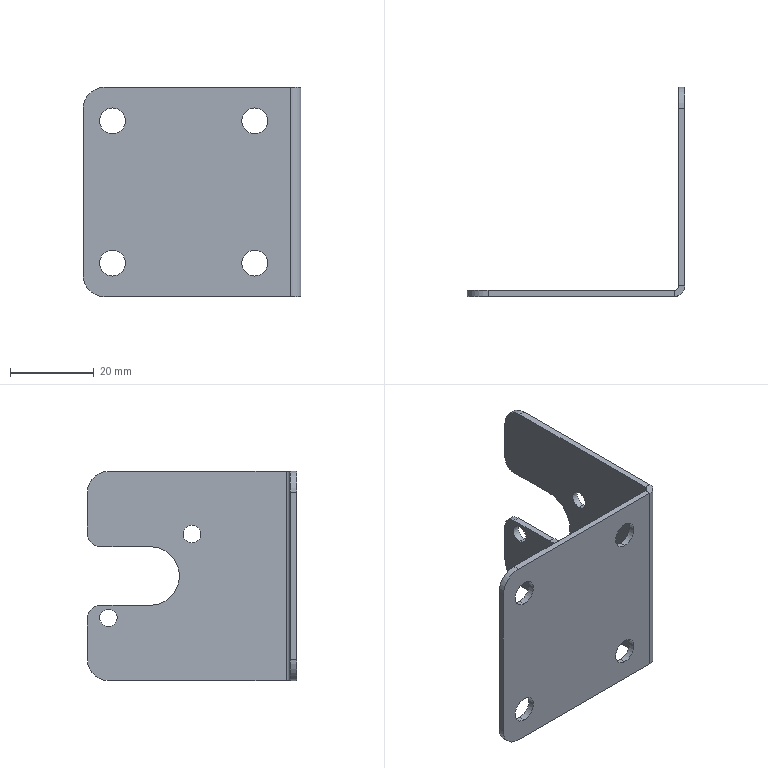Part | SolidWorks | features Fillet 2, HoleWzd 2, ICE 2, EdgeFlange 1, FlatPattern 1, SMBaseFlange 1, SheetMetal 1 | 1 solid | 36 faces | box 52 x 50 x 50 mm | volume 6790 mm3 | cylinder 21 | plane 15 | commonest cylinder face diameters 6.2 x8 4.2 x4 10 x4 6 x2 2 x1 5 x1
STEP:
#1=CARTESIAN_POINT('',(24.5,43.5,-12.1));
#2=VERTEX_POINT('',#1);
#3=CARTESIAN_POINT('',(24.5,43.5,-7.9));
#4=VERTEX_POINT('',#3);
#5=CARTESIAN_POINT('',(24.5,43.5,-10.));
#6=DIRECTION('',(-1.,0.,0.));
#7=DIRECTION('',(0.,-1.,0.));
#8=AXIS2_PLACEMENT_3D('',#5,#6,#7);
#9=CIRCLE('',#8,2.1);
#10=EDGE_CURVE('',#2,#4,#9,.T.);
#11=ORIENTED_EDGE('',*,*,#10,.T.);
#12=CARTESIAN_POINT('',(26.,43.5,-7.9));
#13=VERTEX_POINT('',#12);
#14=CARTESIAN_POINT('',(26.,43.5,-7.9));
#15=DIRECTION('',(1.,0.,0.));
#16=VECTOR('',#15,1000.);
#17=LINE('',#14,#16);
#18=EDGE_CURVE('',#4,#13,#17,.T.);
#19=ORIENTED_EDGE('',*,*,#18,.T.);
#20=CARTESIAN_POINT('',(26.,43.5,-12.1));
#21=VERTEX_POINT('',#20);
#22=CARTESIAN_POINT('',(26.,43.5,-10.));
#23=DIRECTION('',(1.,0.,0.));
#24=DIRECTION('',(0.,0.,-1.));
#25=AXIS2_PLACEMENT_3D('',#22,#23,#24);
#26=CIRCLE('',#25,2.1);
#27=EDGE_CURVE('',#13,#21,#26,.T.);
#28=ORIENTED_EDGE('',*,*,#27,.T.);
#29=CARTESIAN_POINT('',(26.,43.5,-12.1));
#30=DIRECTION('',(1.,0.,0.));
#31=VECTOR('',#30,1000.);
#32=LINE('',#29,#31);
#33=EDGE_CURVE('',#2,#21,#32,.T.);
#34=ORIENTED_EDGE('',*,*,#33,.F.);
#35=EDGE_LOOP('',(#11,#19,#28,#34));
#36=FACE_OUTER_BOUND('',#35,.T.);
#37=CARTESIAN_POINT('',(26.,43.5,-10.));
#38=DIRECTION('',(1.,0.,0.));
#39=DIRECTION('',(0.,0.,-1.));
#40=AXIS2_PLACEMENT_3D('',#37,#38,#39);
#41=CYLINDRICAL_SURFACE('',#40,2.1);
#42=ADVANCED_FACE('',(#36),#41,.F.);
#43=CARTESIAN_POINT('',(24.5,23.5,7.9));
#44=VERTEX_POINT('',#43);
#45=CARTESIAN_POINT('',(24.5,23.5,12.1));
#46=VERTEX_POINT('',#45);
#47=CARTESIAN_POINT('',(24.5,23.5,10.));
#48=DIRECTION('',(-1.,0.,0.));
#49=DIRECTION('',(0.,-1.,0.));
#50=AXIS2_PLACEMENT_3D('',#47,#48,#49);
#51=CIRCLE('',#50,2.1);
#52=EDGE_CURVE('',#44,#46,#51,.T.);
#53=ORIENTED_EDGE('',*,*,#52,.T.);
#54=CARTESIAN_POINT('',(26.,23.5,12.1));
#55=VERTEX_POINT('',#54);
#56=CARTESIAN_POINT('',(26.,23.5,12.1));
#57=DIRECTION('',(1.,0.,0.));
#58=VECTOR('',#57,1000.);
#59=LINE('',#56,#58);
#60=EDGE_CURVE('',#46,#55,#59,.T.);
#61=ORIENTED_EDGE('',*,*,#60,.T.);
#62=CARTESIAN_POINT('',(26.,23.5,7.9));
#63=VERTEX_POINT('',#62);
#64=CARTESIAN_POINT('',(26.,23.5,10.));
#65=DIRECTION('',(1.,0.,0.));
#66=DIRECTION('',(0.,0.,-1.));
#67=AXIS2_PLACEMENT_3D('',#64,#65,#66);
#68=CIRCLE('',#67,2.1);
#69=EDGE_CURVE('',#55,#63,#68,.T.);
#70=ORIENTED_EDGE('',*,*,#69,.T.);
#71=CARTESIAN_POINT('',(26.,23.5,7.9));
#72=DIRECTION('',(1.,0.,0.));
#73=VECTOR('',#72,1000.);
#74=LINE('',#71,#73);
#75=EDGE_CURVE('',#44,#63,#74,.T.);
#76=ORIENTED_EDGE('',*,*,#75,.F.);
#77=EDGE_LOOP('',(#53,#61,#70,#76));
#78=FACE_OUTER_BOUND('',#77,.T.);
#79=CARTESIAN_POINT('',(26.,23.5,10.));
#80=DIRECTION('',(1.,0.,0.));
#81=DIRECTION('',(0.,0.,-1.));
#82=AXIS2_PLACEMENT_3D('',#79,#80,#81);
#83=CYLINDRICAL_SURFACE('',#82,2.1);
#84=ADVANCED_FACE('',(#78),#83,.F.);
#85=CARTESIAN_POINT('',(-19.,-1.5,-13.9));
#86=VERTEX_POINT('',#85);
#87=CARTESIAN_POINT('',(-19.,-1.5,-20.1));
#88=VERTEX_POINT('',#87);
#89=CARTESIAN_POINT('',(-19.,-1.5,-17.));
#90=DIRECTION('',(0.,-1.,0.));
#91=DIRECTION('',(0.,0.,-1.));
#92=AXIS2_PLACEMENT_3D('',#89,#90,#91);
#93=CIRCLE('',#92,3.1);
#94=EDGE_CURVE('',#86,#88,#93,.T.);
#95=ORIENTED_EDGE('',*,*,#94,.T.);
#96=CARTESIAN_POINT('',(-19.,0.,-20.1));
#97=VERTEX_POINT('',#96);
#98=CARTESIAN_POINT('',(-19.,0.,-20.1));
#99=DIRECTION('',(0.,1.,0.));
#100=VECTOR('',#99,1000.);
#101=LINE('',#98,#100);
#102=EDGE_CURVE('',#88,#97,#101,.T.);
#103=ORIENTED_EDGE('',*,*,#102,.T.);
#104=CARTESIAN_POINT('',(-19.,0.,-13.9));
#105=VERTEX_POINT('',#104);
#106=CARTESIAN_POINT('',(-19.,0.,-17.));
#107=DIRECTION('',(0.,1.,0.));
#108=DIRECTION('',(0.,0.,1.));
#109=AXIS2_PLACEMENT_3D('',#106,#107,#108);
#110=CIRCLE('',#109,3.1);
#111=EDGE_CURVE('',#97,#105,#110,.T.);
#112=ORIENTED_EDGE('',*,*,#111,.T.);
#113=CARTESIAN_POINT('',(-19.,0.,-13.9));
#114=DIRECTION('',(0.,1.,0.));
#115=VECTOR('',#114,1000.);
#116=LINE('',#113,#115);
#117=EDGE_CURVE('',#86,#105,#116,.T.);
#118=ORIENTED_EDGE('',*,*,#117,.F.);
#119=EDGE_LOOP('',(#95,#103,#112,#118));
#120=FACE_OUTER_BOUND('',#119,.T.);
#121=CARTESIAN_POINT('',(-19.,0.,-17.));
#122=DIRECTION('',(0.,1.,0.));
#123=DIRECTION('',(0.,0.,1.));
#124=AXIS2_PLACEMENT_3D('',#121,#122,#123);
#125=CYLINDRICAL_SURFACE('',#124,3.1);
#126=ADVANCED_FACE('',(#120),#125,.F.);
#127=CARTESIAN_POINT('',(15.,-1.5,20.1));
#128=VERTEX_POINT('',#127);
#129=CARTESIAN_POINT('',(15.,-1.5,13.9));
#130=VERTEX_POINT('',#129);
#131=CARTESIAN_POINT('',(15.,-1.5,17.));
#132=DIRECTION('',(0.,-1.,0.));
#133=DIRECTION('',(0.,0.,-1.));
#134=AXIS2_PLACEMENT_3D('',#131,#132,#133);
#135=CIRCLE('',#134,3.1);
#136=EDGE_CURVE('',#128,#130,#135,.T.);
#137=ORIENTED_EDGE('',*,*,#136,.T.);
#138=CARTESIAN_POINT('',(15.,0.,13.9));
#139=VERTEX_POINT('',#138);
#140=CARTESIAN_POINT('',(15.,0.,13.9));
#141=DIRECTION('',(0.,1.,0.));
#142=VECTOR('',#141,1000.);
#143=LINE('',#140,#142);
#144=EDGE_CURVE('',#130,#139,#143,.T.);
#145=ORIENTED_EDGE('',*,*,#144,.T.);
#146=CARTESIAN_POINT('',(15.,0.,20.1));
#147=VERTEX_POINT('',#146);
#148=CARTESIAN_POINT('',(15.,0.,17.));
#149=DIRECTION('',(0.,1.,0.));
#150=DIRECTION('',(0.,0.,1.));
#151=AXIS2_PLACEMENT_3D('',#148,#149,#150);
#152=CIRCLE('',#151,3.1);
#153=EDGE_CURVE('',#139,#147,#152,.T.);
#154=ORIENTED_EDGE('',*,*,#153,.T.);
#155=CARTESIAN_POINT('',(15.,0.,20.1));
#156=DIRECTION('',(0.,1.,0.));
#157=VECTOR('',#156,1000.);
#158=LINE('',#155,#157);
#159=EDGE_CURVE('',#128,#147,#158,.T.);
#160=ORIENTED_EDGE('',*,*,#159,.F.);
#161=EDGE_LOOP('',(#137,#145,#154,#160));
#162=FACE_OUTER_BOUND('',#161,.T.);
#163=CARTESIAN_POINT('',(15.,0.,17.));
#164=DIRECTION('',(0.,1.,0.));
#165=DIRECTION('',(0.,0.,1.));
#166=AXIS2_PLACEMENT_3D('',#163,#164,#165);
#167=CYLINDRICAL_SURFACE('',#166,3.1);
#168=ADVANCED_FACE('',(#162),#167,.F.);
#169=CARTESIAN_POINT('',(-19.,-1.5,20.1));
#170=VERTEX_POINT('',#169);
#171=CARTESIAN_POINT('',(-19.,-1.5,13.9));
#172=VERTEX_POINT('',#171);
#173=CARTESIAN_POINT('',(-19.,-1.5,17.));
#174=DIRECTION('',(0.,-1.,0.));
#175=DIRECTION('',(0.,0.,-1.));
#176=AXIS2_PLACEMENT_3D('',#173,#174,#175);
#177=CIRCLE('',#176,3.1);
#178=EDGE_CURVE('',#170,#172,#177,.T.);
#179=ORIENTED_EDGE('',*,*,#178,.T.);
#180=CARTESIAN_POINT('',(-19.,0.,13.9));
#181=VERTEX_POINT('',#180);
#182=CARTESIAN_POINT('',(-19.,0.,13.9));
#183=DIRECTION('',(0.,1.,0.));
#184=VECTOR('',#183,1000.);
#185=LINE('',#182,#184);
#186=EDGE_CURVE('',#172,#181,#185,.T.);
#187=ORIENTED_EDGE('',*,*,#186,.T.);
#188=CARTESIAN_POINT('',(-19.,0.,20.1));
#189=VERTEX_POINT('',#188);
#190=CARTESIAN_POINT('',(-19.,0.,17.));
#191=DIRECTION('',(0.,1.,0.));
#192=DIRECTION('',(0.,0.,1.));
#193=AXIS2_PLACEMENT_3D('',#190,#191,#192);
#194=CIRCLE('',#193,3.1);
#195=EDGE_CURVE('',#181,#189,#194,.T.);
#196=ORIENTED_EDGE('',*,*,#195,.T.);
#197=CARTESIAN_POINT('',(-19.,0.,20.1));
#198=DIRECTION('',(0.,1.,0.));
#199=VECTOR('',#198,1000.);
#200=LINE('',#197,#199);
#201=EDGE_CURVE('',#170,#189,#200,.T.);
#202=ORIENTED_EDGE('',*,*,#201,.F.);
#203=EDGE_LOOP('',(#179,#187,#196,#202));
#204=FACE_OUTER_BOUND('',#203,.T.);
#205=CARTESIAN_POINT('',(-19.,0.,17.));
#206=DIRECTION('',(0.,1.,0.));
#207=DIRECTION('',(0.,0.,1.));
#208=AXIS2_PLACEMENT_3D('',#205,#206,#207);
#209=CYLINDRICAL_SURFACE('',#208,3.1);
#210=ADVANCED_FACE('',(#204),#209,.F.);
#211=CARTESIAN_POINT('',(15.,-1.5,-13.9));
#212=VERTEX_POINT('',#211);
#213=CARTESIAN_POINT('',(15.,-1.5,-20.1));
#214=VERTEX_POINT('',#213);
#215=CARTESIAN_POINT('',(15.,-1.5,-17.));
#216=DIRECTION('',(0.,-1.,0.));
#217=DIRECTION('',(0.,0.,-1.));
#218=AXIS2_PLACEMENT_3D('',#215,#216,#217);
#219=CIRCLE('',#218,3.1);
#220=EDGE_CURVE('',#212,#214,#219,.T.);
#221=ORIENTED_EDGE('',*,*,#220,.T.);
#222=CARTESIAN_POINT('',(15.,0.,-20.1));
#223=VERTEX_POINT('',#222);
#224=CARTESIAN_POINT('',(15.,0.,-20.1));
#225=DIRECTION('',(0.,1.,0.));
#226=VECTOR('',#225,1000.);
#227=LINE('',#224,#226);
#228=EDGE_CURVE('',#214,#223,#227,.T.);
#229=ORIENTED_EDGE('',*,*,#228,.T.);
#230=CARTESIAN_POINT('',(15.,0.,-13.9));
#231=VERTEX_POINT('',#230);
#232=CARTESIAN_POINT('',(15.,0.,-17.));
#233=DIRECTION('',(0.,1.,0.));
#234=DIRECTION('',(0.,0.,1.));
#235=AXIS2_PLACEMENT_3D('',#232,#233,#234);
#236=CIRCLE('',#235,3.1);
#237=EDGE_CURVE('',#223,#231,#236,.T.);
#238=ORIENTED_EDGE('',*,*,#237,.T.);
#239=CARTESIAN_POINT('',(15.,0.,-13.9));
#240=DIRECTION('',(0.,1.,0.));
#241=VECTOR('',#240,1000.);
#242=LINE('',#239,#241);
#243=EDGE_CURVE('',#212,#231,#242,.T.);
#244=ORIENTED_EDGE('',*,*,#243,.F.);
#245=EDGE_LOOP('',(#221,#229,#238,#244));
#246=FACE_OUTER_BOUND('',#245,.T.);
#247=CARTESIAN_POINT('',(15.,0.,-17.));
#248=DIRECTION('',(0.,1.,0.));
#249=DIRECTION('',(0.,0.,1.));
#250=AXIS2_PLACEMENT_3D('',#247,#248,#249);
#251=CYLINDRICAL_SURFACE('',#250,3.1);
#252=ADVANCED_FACE('',(#246),#251,.F.);
#253=CARTESIAN_POINT('',(26.,23.5,10.));
#254=DIRECTION('',(1.,0.,0.));
#255=DIRECTION('',(0.,0.,-1.));
#256=AXIS2_PLACEMENT_3D('',#253,#254,#255);
#257=CIRCLE('',#256,2.1);
#258=EDGE_CURVE('',#63,#55,#257,.T.);
#259=ORIENTED_EDGE('',*,*,#258,.F.);
#260=ORIENTED_EDGE('',*,*,#69,.F.);
#261=EDGE_LOOP('',(#259,#260));
#262=FACE_BOUND('',#261,.T.);
#263=CARTESIAN_POINT('',(26.,43.5,-10.));
#264=DIRECTION('',(1.,0.,0.));
#265=DIRECTION('',(0.,0.,-1.));
#266=AXIS2_PLACEMENT_3D('',#263,#264,#265);
#267=CIRCLE('',#266,2.1);
#268=EDGE_CURVE('',#21,#13,#267,.T.);
#269=ORIENTED_EDGE('',*,*,#268,.F.);
#270=ORIENTED_EDGE('',*,*,#27,.F.);
#271=EDGE_LOOP('',(#269,#270));
#272=FACE_BOUND('',#271,.T.);
#273=CARTESIAN_POINT('',(26.,33.5,7.));
#274=VERTEX_POINT('',#273);
#275=CARTESIAN_POINT('',(26.,45.5,7.));
#276=VERTEX_POINT('',#275);
#277=CARTESIAN_POINT('',(26.,0.,7.));
#278=DIRECTION('',(0.,1.,0.));
#279=VECTOR('',#278,1000.);
#280=LINE('',#277,#279);
#281=EDGE_CURVE('',#274,#276,#280,.T.);
#282=ORIENTED_EDGE('',*,*,#281,.T.);
#283=CARTESIAN_POINT('',(26.,48.5,10.));
#284=VERTEX_POINT('',#283);
#285=CARTESIAN_POINT('',(26.,45.5,10.));
#286=DIRECTION('',(1.,0.,0.));
#287=DIRECTION('',(0.,-1.,0.));
#288=AXIS2_PLACEMENT_3D('',#285,#286,#287);
#289=CIRCLE('',#288,3.);
#290=EDGE_CURVE('',#276,#284,#289,.T.);
#291=ORIENTED_EDGE('',*,*,#290,.T.);
#292=CARTESIAN_POINT('',(26.,48.5,20.));
#293=VERTEX_POINT('',#292);
#294=CARTESIAN_POINT('',(26.,48.5,0.));
#295=DIRECTION('',(0.,0.,1.));
#296=VECTOR('',#295,1000.);
#297=LINE('',#294,#296);
#298=EDGE_CURVE('',#284,#293,#297,.T.);
#299=ORIENTED_EDGE('',*,*,#298,.T.);
#300=CARTESIAN_POINT('',(26.,43.5,25.));
#301=VERTEX_POINT('',#300);
#302=CARTESIAN_POINT('',(26.,43.5,20.));
#303=DIRECTION('',(1.,0.,0.));
#304=DIRECTION('',(0.,-1.,0.));
#305=AXIS2_PLACEMENT_3D('',#302,#303,#304);
#306=CIRCLE('',#305,5.);
#307=EDGE_CURVE('',#293,#301,#306,.T.);
#308=ORIENTED_EDGE('',*,*,#307,.T.);
#309=CARTESIAN_POINT('',(26.,1.,25.));
#310=VERTEX_POINT('',#309);
#311=CARTESIAN_POINT('',(26.,0.,25.));
#312=DIRECTION('',(0.,-1.,0.));
#313=VECTOR('',#312,1000.);
#314=LINE('',#311,#313);
#315=EDGE_CURVE('',#301,#310,#314,.T.);
#316=ORIENTED_EDGE('',*,*,#315,.T.);
#317=CARTESIAN_POINT('',(26.,1.,-25.));
#318=VERTEX_POINT('',#317);
#319=CARTESIAN_POINT('',(26.,1.,25.));
#320=DIRECTION('',(0.,0.,1.));
#321=VECTOR('',#320,1000.);
#322=LINE('',#319,#321);
#323=EDGE_CURVE('',#318,#310,#322,.T.);
#324=ORIENTED_EDGE('',*,*,#323,.F.);
#325=CARTESIAN_POINT('',(26.,43.5,-25.));
#326=VERTEX_POINT('',#325);
#327=CARTESIAN_POINT('',(26.,0.,-25.));
#328=DIRECTION('',(0.,1.,0.));
#329=VECTOR('',#328,1000.);
#330=LINE('',#327,#329);
#331=EDGE_CURVE('',#318,#326,#330,.T.);
#332=ORIENTED_EDGE('',*,*,#331,.T.);
#333=CARTESIAN_POINT('',(26.,48.5,-20.));
#334=VERTEX_POINT('',#333);
#335=CARTESIAN_POINT('',(26.,43.5,-20.));
#336=DIRECTION('',(1.,0.,0.));
#337=DIRECTION('',(0.,-1.,0.));
#338=AXIS2_PLACEMENT_3D('',#335,#336,#337);
#339=CIRCLE('',#338,5.);
#340=EDGE_CURVE('',#326,#334,#339,.T.);
#341=ORIENTED_EDGE('',*,*,#340,.T.);
#342=CARTESIAN_POINT('',(26.,48.5,-10.));
#343=VERTEX_POINT('',#342);
#344=CARTESIAN_POINT('',(26.,48.5,0.));
#345=DIRECTION('',(0.,0.,1.));
#346=VECTOR('',#345,1000.);
#347=LINE('',#344,#346);
#348=EDGE_CURVE('',#334,#343,#347,.T.);
#349=ORIENTED_EDGE('',*,*,#348,.T.);
#350=CARTESIAN_POINT('',(26.,45.5,-7.));
#351=VERTEX_POINT('',#350);
#352=CARTESIAN_POINT('',(26.,45.5,-10.));
#353=DIRECTION('',(1.,0.,0.));
#354=DIRECTION('',(0.,-1.,0.));
#355=AXIS2_PLACEMENT_3D('',#352,#353,#354);
#356=CIRCLE('',#355,3.);
#357=EDGE_CURVE('',#343,#351,#356,.T.);
#358=ORIENTED_EDGE('',*,*,#357,.T.);
#359=CARTESIAN_POINT('',(26.,33.5,-7.));
#360=VERTEX_POINT('',#359);
#361=CARTESIAN_POINT('',(26.,0.,-7.));
#362=DIRECTION('',(0.,-1.,0.));
#363=VECTOR('',#362,1000.);
#364=LINE('',#361,#363);
#365=EDGE_CURVE('',#351,#360,#364,.T.);
#366=ORIENTED_EDGE('',*,*,#365,.T.);
#367=CARTESIAN_POINT('',(26.,33.5,0.));
#368=DIRECTION('',(1.,0.,0.));
#369=DIRECTION('',(0.,1.,0.));
#370=AXIS2_PLACEMENT_3D('',#367,#368,#369);
#371=CIRCLE('',#370,7.);
#372=EDGE_CURVE('',#274,#360,#371,.T.);
#373=ORIENTED_EDGE('',*,*,#372,.F.);
#374=EDGE_LOOP('',(#282,#291,#299,#308,#316,#324,#332,#341,#349,#358,#366,#373));
#375=FACE_OUTER_BOUND('',#374,.T.);
#376=CARTESIAN_POINT('',(26.,0.,0.));
#377=DIRECTION('',(-1.,0.,0.));
#378=DIRECTION('',(0.,-1.,0.));
#379=AXIS2_PLACEMENT_3D('',#376,#377,#378);
#380=PLANE('',#379);
#381=ADVANCED_FACE('',(#262,#272,#375),#380,.F.);
#382=ORIENTED_EDGE('',*,*,#10,.F.);
#383=CARTESIAN_POINT('',(24.5,43.5,-10.));
#384=DIRECTION('',(-1.,0.,0.));
#385=DIRECTION('',(0.,-1.,0.));
#386=AXIS2_PLACEMENT_3D('',#383,#384,#385);
#387=CIRCLE('',#386,2.1);
#388=EDGE_CURVE('',#4,#2,#387,.T.);
#389=ORIENTED_EDGE('',*,*,#388,.F.);
#390=EDGE_LOOP('',(#382,#389));
#391=FACE_BOUND('',#390,.T.);
#392=ORIENTED_EDGE('',*,*,#52,.F.);
#393=CARTESIAN_POINT('',(24.5,23.5,10.));
#394=DIRECTION('',(-1.,0.,0.));
#395=DIRECTION('',(0.,-1.,0.));
#396=AXIS2_PLACEMENT_3D('',#393,#394,#395);
#397=CIRCLE('',#396,2.1);
#398=EDGE_CURVE('',#46,#44,#397,.T.);
#399=ORIENTED_EDGE('',*,*,#398,.F.);
#400=EDGE_LOOP('',(#392,#399));
#401=FACE_BOUND('',#400,.T.);
#402=CARTESIAN_POINT('',(24.5,48.5,10.));
#403=VERTEX_POINT('',#402);
#404=CARTESIAN_POINT('',(24.5,48.5,20.));
#405=VERTEX_POINT('',#404);
#406=CARTESIAN_POINT('',(24.5,48.5,25.));
#407=DIRECTION('',(0.,0.,1.));
#408=VECTOR('',#407,1000.);
#409=LINE('',#406,#408);
#410=EDGE_CURVE('',#403,#405,#409,.T.);
#411=ORIENTED_EDGE('',*,*,#410,.F.);
#412=CARTESIAN_POINT('',(24.5,45.5,7.));
#413=VERTEX_POINT('',#412);
#414=CARTESIAN_POINT('',(24.5,45.5,10.));
#415=DIRECTION('',(-1.,0.,0.));
#416=DIRECTION('',(0.,-1.,0.));
#417=AXIS2_PLACEMENT_3D('',#414,#415,#416);
#418=CIRCLE('',#417,3.);
#419=EDGE_CURVE('',#403,#413,#418,.T.);
#420=ORIENTED_EDGE('',*,*,#419,.T.);
#421=CARTESIAN_POINT('',(24.5,33.5,7.));
#422=VERTEX_POINT('',#421);
#423=CARTESIAN_POINT('',(24.5,0.,7.));
#424=DIRECTION('',(0.,1.,0.));
#425=VECTOR('',#424,1000.);
#426=LINE('',#423,#425);
#427=EDGE_CURVE('',#422,#413,#426,.T.);
#428=ORIENTED_EDGE('',*,*,#427,.F.);
#429=CARTESIAN_POINT('',(24.5,33.5,-7.));
#430=VERTEX_POINT('',#429);
#431=CARTESIAN_POINT('',(24.5,33.5,0.));
#432=DIRECTION('',(-1.,0.,0.));
#433=DIRECTION('',(0.,-1.,0.));
#434=AXIS2_PLACEMENT_3D('',#431,#432,#433);
#435=CIRCLE('',#434,7.);
#436=EDGE_CURVE('',#430,#422,#435,.T.);
#437=ORIENTED_EDGE('',*,*,#436,.F.);
#438=CARTESIAN_POINT('',(24.5,45.5,-7.));
#439=VERTEX_POINT('',#438);
#440=CARTESIAN_POINT('',(24.5,0.,-7.));
#441=DIRECTION('',(0.,-1.,0.));
#442=VECTOR('',#441,1000.);
#443=LINE('',#440,#442);
#444=EDGE_CURVE('',#439,#430,#443,.T.);
#445=ORIENTED_EDGE('',*,*,#444,.F.);
#446=CARTESIAN_POINT('',(24.5,48.5,-10.));
#447=VERTEX_POINT('',#446);
#448=CARTESIAN_POINT('',(24.5,45.5,-10.));
#449=DIRECTION('',(-1.,0.,0.));
#450=DIRECTION('',(0.,-1.,0.));
#451=AXIS2_PLACEMENT_3D('',#448,#449,#450);
#452=CIRCLE('',#451,3.);
#453=EDGE_CURVE('',#439,#447,#452,.T.);
#454=ORIENTED_EDGE('',*,*,#453,.T.);
#455=CARTESIAN_POINT('',(24.5,48.5,-20.));
#456=VERTEX_POINT('',#455);
#457=CARTESIAN_POINT('',(24.5,48.5,25.));
#458=DIRECTION('',(0.,0.,1.));
#459=VECTOR('',#458,1000.);
#460=LINE('',#457,#459);
#461=EDGE_CURVE('',#456,#447,#460,.T.);
#462=ORIENTED_EDGE('',*,*,#461,.F.);
#463=CARTESIAN_POINT('',(24.5,43.5,-25.));
#464=VERTEX_POINT('',#463);
#465=CARTESIAN_POINT('',(24.5,43.5,-20.));
#466=DIRECTION('',(-1.,0.,0.));
#467=DIRECTION('',(0.,-1.,0.));
#468=AXIS2_PLACEMENT_3D('',#465,#466,#467);
#469=CIRCLE('',#468,5.);
#470=EDGE_CURVE('',#456,#464,#469,.T.);
#471=ORIENTED_EDGE('',*,*,#470,.T.);
#472=CARTESIAN_POINT('',(24.5,1.,-25.));
#473=VERTEX_POINT('',#472);
#474=CARTESIAN_POINT('',(24.5,48.5,-25.));
#475=DIRECTION('',(0.,1.,0.));
#476=VECTOR('',#475,1000.);
#477=LINE('',#474,#476);
#478=EDGE_CURVE('',#473,#464,#477,.T.);
#479=ORIENTED_EDGE('',*,*,#478,.F.);
#480=CARTESIAN_POINT('',(24.5,1.,25.));
#481=VERTEX_POINT('',#480);
#482=CARTESIAN_POINT('',(24.5,1.,25.));
#483=DIRECTION('',(0.,0.,-1.));
#484=VECTOR('',#483,1000.);
#485=LINE('',#482,#484);
#486=EDGE_CURVE('',#481,#473,#485,.T.);
#487=ORIENTED_EDGE('',*,*,#486,.F.);
#488=CARTESIAN_POINT('',(24.5,43.5,25.));
#489=VERTEX_POINT('',#488);
#490=CARTESIAN_POINT('',(24.5,0.,25.));
#491=DIRECTION('',(0.,-1.,0.));
#492=VECTOR('',#491,1000.);
#493=LINE('',#490,#492);
#494=EDGE_CURVE('',#489,#481,#493,.T.);
#495=ORIENTED_EDGE('',*,*,#494,.F.);
#496=CARTESIAN_POINT('',(24.5,43.5,20.));
#497=DIRECTION('',(-1.,0.,0.));
#498=DIRECTION('',(0.,-1.,0.));
#499=AXIS2_PLACEMENT_3D('',#496,#497,#498);
#500=CIRCLE('',#499,5.);
#501=EDGE_CURVE('',#489,#405,#500,.T.);
#502=ORIENTED_EDGE('',*,*,#501,.T.);
#503=EDGE_LOOP('',(#411,#420,#428,#437,#445,#454,#462,#471,#479,#487,#495,#502));
#504=FACE_OUTER_BOUND('',#503,.T.);
#505=CARTESIAN_POINT('',(24.5,0.,0.));
#506=DIRECTION('',(-1.,0.,0.));
#507=DIRECTION('',(0.,-1.,0.));
#508=AXIS2_PLACEMENT_3D('',#505,#506,#507);
#509=PLANE('',#508);
#510=ADVANCED_FACE('',(#391,#401,#504),#509,.T.);
#511=ORIENTED_EDGE('',*,*,#461,.T.);
#512=CARTESIAN_POINT('',(26.,48.5,-10.));
#513=DIRECTION('',(1.,0.,0.));
#514=VECTOR('',#513,1000.);
#515=LINE('',#512,#514);
#516=EDGE_CURVE('',#447,#343,#515,.T.);
#517=ORIENTED_EDGE('',*,*,#516,.T.);
#518=ORIENTED_EDGE('',*,*,#348,.F.);
#519=CARTESIAN_POINT('',(26.,48.5,-20.));
#520=DIRECTION('',(-1.,0.,0.));
#521=VECTOR('',#520,1000.);
#522=LINE('',#519,#521);
#523=EDGE_CURVE('',#334,#456,#522,.T.);
#524=ORIENTED_EDGE('',*,*,#523,.T.);
#525=EDGE_LOOP('',(#511,#517,#518,#524));
#526=FACE_OUTER_BOUND('',#525,.T.);
#527=CARTESIAN_POINT('',(26.,48.5,25.));
#528=DIRECTION('',(0.,-1.,0.));
#529=DIRECTION('',(1.,0.,0.));
#530=AXIS2_PLACEMENT_3D('',#527,#528,#529);
#531=PLANE('',#530);
#532=ADVANCED_FACE('',(#526),#531,.F.);
#533=ORIENTED_EDGE('',*,*,#298,.F.);
#534=CARTESIAN_POINT('',(24.5,48.5,10.));
#535=DIRECTION('',(-1.,0.,0.));
#536=VECTOR('',#535,1000.);
#537=LINE('',#534,#536);
#538=EDGE_CURVE('',#284,#403,#537,.T.);
#539=ORIENTED_EDGE('',*,*,#538,.T.);
#540=ORIENTED_EDGE('',*,*,#410,.T.);
#541=CARTESIAN_POINT('',(26.,48.5,20.));
#542=DIRECTION('',(1.,0.,0.));
#543=VECTOR('',#542,1000.);
#544=LINE('',#541,#543);
#545=EDGE_CURVE('',#405,#293,#544,.T.);
#546=ORIENTED_EDGE('',*,*,#545,.T.);
#547=EDGE_LOOP('',(#533,#539,#540,#546));
#548=FACE_OUTER_BOUND('',#547,.T.);
#549=CARTESIAN_POINT('',(26.,48.5,25.));
#550=DIRECTION('',(0.,-1.,0.));
#551=DIRECTION('',(1.,0.,0.));
#552=AXIS2_PLACEMENT_3D('',#549,#550,#551);
#553=PLANE('',#552);
#554=ADVANCED_FACE('',(#548),#553,.F.);
#555=CARTESIAN_POINT('',(24.5,33.5,-7.));
#556=DIRECTION('',(1.,0.,0.));
#557=VECTOR('',#556,1000.);
#558=LINE('',#555,#557);
#559=EDGE_CURVE('',#430,#360,#558,.T.);
#560=ORIENTED_EDGE('',*,*,#559,.F.);
#561=ORIENTED_EDGE('',*,*,#436,.T.);
#562=CARTESIAN_POINT('',(24.5,33.5,7.));
#563=DIRECTION('',(1.,0.,0.));
#564=VECTOR('',#563,1000.);
#565=LINE('',#562,#564);
#566=EDGE_CURVE('',#422,#274,#565,.T.);
#567=ORIENTED_EDGE('',*,*,#566,.T.);
#568=ORIENTED_EDGE('',*,*,#372,.T.);
#569=EDGE_LOOP('',(#560,#561,#567,#568));
#570=FACE_OUTER_BOUND('',#569,.T.);
#571=CARTESIAN_POINT('',(-26.,33.5,0.));
#572=DIRECTION('',(1.,0.,0.));
#573=DIRECTION('',(0.,1.,0.));
#574=AXIS2_PLACEMENT_3D('',#571,#572,#573);
#575=CYLINDRICAL_SURFACE('',#574,7.);
#576=ADVANCED_FACE('',(#570),#575,.F.);
#577=CARTESIAN_POINT('',(23.5,-1.5,-25.));
#578=VERTEX_POINT('',#577);
#579=CARTESIAN_POINT('',(-21.,-1.5,-25.));
#580=VERTEX_POINT('',#579);
#581=CARTESIAN_POINT('',(-26.,-1.5,-25.));
#582=DIRECTION('',(-1.,0.,0.));
#583=VECTOR('',#582,1000.);
#584=LINE('',#581,#583);
#585=EDGE_CURVE('',#578,#580,#584,.T.);
#586=ORIENTED_EDGE('',*,*,#585,.T.);
#587=CARTESIAN_POINT('',(-21.,0.,-25.));
#588=VERTEX_POINT('',#587);
#589=CARTESIAN_POINT('',(-21.,-1.5,-25.));
#590=DIRECTION('',(0.,1.,0.));
#591=VECTOR('',#590,1000.);
#592=LINE('',#589,#591);
#593=EDGE_CURVE('',#580,#588,#592,.T.);
#594=ORIENTED_EDGE('',*,*,#593,.T.);
#595=CARTESIAN_POINT('',(23.5,0.,-25.));
#596=VERTEX_POINT('',#595);
#597=CARTESIAN_POINT('',(-26.,0.,-25.));
#598=DIRECTION('',(-1.,0.,0.));
#599=VECTOR('',#598,1000.);
#600=LINE('',#597,#599);
#601=EDGE_CURVE('',#596,#588,#600,.T.);
#602=ORIENTED_EDGE('',*,*,#601,.F.);
#603=CARTESIAN_POINT('',(23.5,0.,-25.));
#604=DIRECTION('',(0.,-1.,0.));
#605=VECTOR('',#604,1000.);
#606=LINE('',#603,#605);
#607=EDGE_CURVE('',#596,#578,#606,.T.);
#608=ORIENTED_EDGE('',*,*,#607,.T.);
#609=EDGE_LOOP('',(#586,#594,#602,#608));
#610=FACE_OUTER_BOUND('',#609,.T.);
#611=CARTESIAN_POINT('',(-26.,-1.5,-25.));
#612=DIRECTION('',(0.,0.,-1.));
#613=DIRECTION('',(-1.,0.,0.));
#614=AXIS2_PLACEMENT_3D('',#611,#612,#613);
#615=PLANE('',#614);
#616=ADVANCED_FACE('',(#610),#615,.T.);
#617=ORIENTED_EDGE('',*,*,#94,.F.);
#618=CARTESIAN_POINT('',(-19.,-1.5,-17.));
#619=DIRECTION('',(0.,-1.,0.));
#620=DIRECTION('',(0.,0.,-1.));
#621=AXIS2_PLACEMENT_3D('',#618,#619,#620);
#622=CIRCLE('',#621,3.1);
#623=EDGE_CURVE('',#88,#86,#622,.T.);
#624=ORIENTED_EDGE('',*,*,#623,.F.);
#625=EDGE_LOOP('',(#617,#624));
#626=FACE_BOUND('',#625,.T.);
#627=ORIENTED_EDGE('',*,*,#136,.F.);
#628=CARTESIAN_POINT('',(15.,-1.5,17.));
#629=DIRECTION('',(0.,-1.,0.));
#630=DIRECTION('',(0.,0.,-1.));
#631=AXIS2_PLACEMENT_3D('',#628,#629,#630);
#632=CIRCLE('',#631,3.1);
#633=EDGE_CURVE('',#130,#128,#632,.T.);
#634=ORIENTED_EDGE('',*,*,#633,.F.);
#635=EDGE_LOOP('',(#627,#634));
#636=FACE_BOUND('',#635,.T.);
#637=ORIENTED_EDGE('',*,*,#178,.F.);
#638=CARTESIAN_POINT('',(-19.,-1.5,17.));
#639=DIRECTION('',(0.,-1.,0.));
#640=DIRECTION('',(0.,0.,-1.));
#641=AXIS2_PLACEMENT_3D('',#638,#639,#640);
#642=CIRCLE('',#641,3.1);
#643=EDGE_CURVE('',#172,#170,#642,.T.);
#644=ORIENTED_EDGE('',*,*,#643,.F.);
#645=EDGE_LOOP('',(#637,#644));
#646=FACE_BOUND('',#645,.T.);
#647=ORIENTED_EDGE('',*,*,#220,.F.);
#648=CARTESIAN_POINT('',(15.,-1.5,-17.));
#649=DIRECTION('',(0.,-1.,0.));
#650=DIRECTION('',(0.,0.,-1.));
#651=AXIS2_PLACEMENT_3D('',#648,#649,#650);
#652=CIRCLE('',#651,3.1);
#653=EDGE_CURVE('',#214,#212,#652,.T.);
#654=ORIENTED_EDGE('',*,*,#653,.F.);
#655=EDGE_LOOP('',(#647,#654));
#656=FACE_BOUND('',#655,.T.);
#657=CARTESIAN_POINT('',(-21.,-1.5,25.));
#658=VERTEX_POINT('',#657);
#659=CARTESIAN_POINT('',(23.5,-1.5,25.));
#660=VERTEX_POINT('',#659);
#661=CARTESIAN_POINT('',(-26.,-1.5,25.));
#662=DIRECTION('',(1.,0.,0.));
#663=VECTOR('',#662,1000.);
#664=LINE('',#661,#663);
#665=EDGE_CURVE('',#658,#660,#664,.T.);
#666=ORIENTED_EDGE('',*,*,#665,.F.);
#667=CARTESIAN_POINT('',(-26.,-1.5,20.));
#668=VERTEX_POINT('',#667);
#669=CARTESIAN_POINT('',(-21.,-1.5,20.));
#670=DIRECTION('',(0.,-1.,0.));
#671=DIRECTION('',(0.,0.,-1.));
#672=AXIS2_PLACEMENT_3D('',#669,#670,#671);
#673=CIRCLE('',#672,5.);
#674=EDGE_CURVE('',#658,#668,#673,.T.);
#675=ORIENTED_EDGE('',*,*,#674,.T.);
#676=CARTESIAN_POINT('',(-26.,-1.5,-20.));
#677=VERTEX_POINT('',#676);
#678=CARTESIAN_POINT('',(-26.,-1.5,25.));
#679=DIRECTION('',(0.,0.,1.));
#680=VECTOR('',#679,1000.);
#681=LINE('',#678,#680);
#682=EDGE_CURVE('',#677,#668,#681,.T.);
#683=ORIENTED_EDGE('',*,*,#682,.F.);
#684=CARTESIAN_POINT('',(-21.,-1.5,-20.));
#685=DIRECTION('',(0.,-1.,0.));
#686=DIRECTION('',(0.,0.,-1.));
#687=AXIS2_PLACEMENT_3D('',#684,#685,#686);
#688=CIRCLE('',#687,5.);
#689=EDGE_CURVE('',#677,#580,#688,.T.);
#690=ORIENTED_EDGE('',*,*,#689,.T.);
#691=ORIENTED_EDGE('',*,*,#585,.F.);
#692=CARTESIAN_POINT('',(23.5,-1.5,-25.));
#693=DIRECTION('',(0.,0.,1.));
#694=VECTOR('',#693,1000.);
#695=LINE('',#692,#694);
#696=EDGE_CURVE('',#578,#660,#695,.T.);
#697=ORIENTED_EDGE('',*,*,#696,.T.);
#698=EDGE_LOOP('',(#666,#675,#683,#690,#691,#697));
#699=FACE_OUTER_BOUND('',#698,.T.);
#700=CARTESIAN_POINT('',(0.,-1.5,0.));
#701=DIRECTION('',(0.,-1.,0.));
#702=DIRECTION('',(0.,0.,-1.));
#703=AXIS2_PLACEMENT_3D('',#700,#701,#702);
#704=PLANE('',#703);
#705=ADVANCED_FACE('',(#626,#636,#646,#656,#699),#704,.T.);
#706=CARTESIAN_POINT('',(-19.,0.,-17.));
#707=DIRECTION('',(0.,1.,0.));
#708=DIRECTION('',(0.,0.,1.));
#709=AXIS2_PLACEMENT_3D('',#706,#707,#708);
#710=CIRCLE('',#709,3.1);
#711=EDGE_CURVE('',#105,#97,#710,.T.);
#712=ORIENTED_EDGE('',*,*,#711,.F.);
#713=ORIENTED_EDGE('',*,*,#111,.F.);
#714=EDGE_LOOP('',(#712,#713));
#715=FACE_BOUND('',#714,.T.);
#716=CARTESIAN_POINT('',(15.,0.,17.));
#717=DIRECTION('',(0.,1.,0.));
#718=DIRECTION('',(0.,0.,1.));
#719=AXIS2_PLACEMENT_3D('',#716,#717,#718);
#720=CIRCLE('',#719,3.1);
#721=EDGE_CURVE('',#147,#139,#720,.T.);
#722=ORIENTED_EDGE('',*,*,#721,.F.);
#723=ORIENTED_EDGE('',*,*,#153,.F.);
#724=EDGE_LOOP('',(#722,#723));
#725=FACE_BOUND('',#724,.T.);
#726=CARTESIAN_POINT('',(-19.,0.,17.));
#727=DIRECTION('',(0.,1.,0.));
#728=DIRECTION('',(0.,0.,1.));
#729=AXIS2_PLACEMENT_3D('',#726,#727,#728);
#730=CIRCLE('',#729,3.1);
#731=EDGE_CURVE('',#189,#181,#730,.T.);
#732=ORIENTED_EDGE('',*,*,#731,.F.);
#733=ORIENTED_EDGE('',*,*,#195,.F.);
#734=EDGE_LOOP('',(#732,#733));
#735=FACE_BOUND('',#734,.T.);
#736=CARTESIAN_POINT('',(15.,0.,-17.));
#737=DIRECTION('',(0.,1.,0.));
#738=DIRECTION('',(0.,0.,1.));
#739=AXIS2_PLACEMENT_3D('',#736,#737,#738);
#740=CIRCLE('',#739,3.1);
#741=EDGE_CURVE('',#231,#223,#740,.T.);
#742=ORIENTED_EDGE('',*,*,#741,.F.);
#743=ORIENTED_EDGE('',*,*,#237,.F.);
#744=EDGE_LOOP('',(#742,#743));
#745=FACE_BOUND('',#744,.T.);
#746=CARTESIAN_POINT('',(-26.,0.,-20.));
#747=VERTEX_POINT('',#746);
#748=CARTESIAN_POINT('',(-26.,0.,20.));
#749=VERTEX_POINT('',#748);
#750=CARTESIAN_POINT('',(-26.,0.,25.));
#751=DIRECTION('',(0.,0.,1.));
#752=VECTOR('',#751,1000.);
#753=LINE('',#750,#752);
#754=EDGE_CURVE('',#747,#749,#753,.T.);
#755=ORIENTED_EDGE('',*,*,#754,.T.);
#756=CARTESIAN_POINT('',(-21.,0.,25.));
#757=VERTEX_POINT('',#756);
#758=CARTESIAN_POINT('',(-21.,0.,20.));
#759=DIRECTION('',(0.,1.,0.));
#760=DIRECTION('',(0.,0.,-1.));
#761=AXIS2_PLACEMENT_3D('',#758,#759,#760);
#762=CIRCLE('',#761,5.);
#763=EDGE_CURVE('',#749,#757,#762,.T.);
#764=ORIENTED_EDGE('',*,*,#763,.T.);
#765=CARTESIAN_POINT('',(23.5,0.,25.));
#766=VERTEX_POINT('',#765);
#767=CARTESIAN_POINT('',(-26.,0.,25.));
#768=DIRECTION('',(1.,0.,0.));
#769=VECTOR('',#768,1000.);
#770=LINE('',#767,#769);
#771=EDGE_CURVE('',#757,#766,#770,.T.);
#772=ORIENTED_EDGE('',*,*,#771,.T.);
#773=CARTESIAN_POINT('',(23.5,0.,-25.));
#774=DIRECTION('',(0.,0.,1.));
#775=VECTOR('',#774,1000.);
#776=LINE('',#773,#775);
#777=EDGE_CURVE('',#596,#766,#776,.T.);
#778=ORIENTED_EDGE('',*,*,#777,.F.);
#779=ORIENTED_EDGE('',*,*,#601,.T.);
#780=CARTESIAN_POINT('',(-21.,0.,-20.));
#781=DIRECTION('',(0.,1.,0.));
#782=DIRECTION('',(0.,0.,-1.));
#783=AXIS2_PLACEMENT_3D('',#780,#781,#782);
#784=CIRCLE('',#783,5.);
#785=EDGE_CURVE('',#588,#747,#784,.T.);
#786=ORIENTED_EDGE('',*,*,#785,.T.);
#787=EDGE_LOOP('',(#755,#764,#772,#778,#779,#786));
#788=FACE_OUTER_BOUND('',#787,.T.);
#789=CARTESIAN_POINT('',(0.,0.,0.));
#790=DIRECTION('',(0.,-1.,0.));
#791=DIRECTION('',(0.,0.,-1.));
#792=AXIS2_PLACEMENT_3D('',#789,#790,#791);
#793=PLANE('',#792);
#794=ADVANCED_FACE('',(#715,#725,#735,#745,#788),#793,.F.);
#795=ORIENTED_EDGE('',*,*,#771,.F.);
#796=CARTESIAN_POINT('',(-21.,-1.5,25.));
#797=DIRECTION('',(0.,-1.,0.));
#798=VECTOR('',#797,1000.);
#799=LINE('',#796,#798);
#800=EDGE_CURVE('',#757,#658,#799,.T.);
#801=ORIENTED_EDGE('',*,*,#800,.T.);
#802=ORIENTED_EDGE('',*,*,#665,.T.);
#803=CARTESIAN_POINT('',(23.5,0.,25.));
#804=DIRECTION('',(0.,-1.,0.));
#805=VECTOR('',#804,1000.);
#806=LINE('',#803,#805);
#807=EDGE_CURVE('',#766,#660,#806,.T.);
#808=ORIENTED_EDGE('',*,*,#807,.F.);
#809=EDGE_LOOP('',(#795,#801,#802,#808));
#810=FACE_OUTER_BOUND('',#809,.T.);
#811=CARTESIAN_POINT('',(-26.,-1.5,25.));
#812=DIRECTION('',(0.,0.,1.));
#813=DIRECTION('',(1.,0.,0.));
#814=AXIS2_PLACEMENT_3D('',#811,#812,#813);
#815=PLANE('',#814);
#816=ADVANCED_FACE('',(#810),#815,.T.);
#817=ORIENTED_EDGE('',*,*,#682,.T.);
#818=CARTESIAN_POINT('',(-26.,-1.5,20.));
#819=DIRECTION('',(0.,1.,0.));
#820=VECTOR('',#819,1000.);
#821=LINE('',#818,#820);
#822=EDGE_CURVE('',#668,#749,#821,.T.);
#823=ORIENTED_EDGE('',*,*,#822,.T.);
#824=ORIENTED_EDGE('',*,*,#754,.F.);
#825=CARTESIAN_POINT('',(-26.,-1.5,-20.));
#826=DIRECTION('',(0.,-1.,0.));
#827=VECTOR('',#826,1000.);
#828=LINE('',#825,#827);
#829=EDGE_CURVE('',#747,#677,#828,.T.);
#830=ORIENTED_EDGE('',*,*,#829,.T.);
#831=EDGE_LOOP('',(#817,#823,#824,#830));
#832=FACE_OUTER_BOUND('',#831,.T.);
#833=CARTESIAN_POINT('',(-26.,-1.5,25.));
#834=DIRECTION('',(-1.,0.,0.));
#835=DIRECTION('',(0.,0.,1.));
#836=AXIS2_PLACEMENT_3D('',#833,#834,#835);
#837=PLANE('',#836);
#838=ADVANCED_FACE('',(#832),#837,.T.);
#839=CARTESIAN_POINT('',(26.,1.,25.));
#840=DIRECTION('',(1.,0.,0.));
#841=VECTOR('',#840,1000.);
#842=LINE('',#839,#841);
#843=EDGE_CURVE('',#481,#310,#842,.T.);
#844=ORIENTED_EDGE('',*,*,#843,.F.);
#845=CARTESIAN_POINT('',(23.5,1.,25.));
#846=DIRECTION('',(0.,0.,1.));
#847=DIRECTION('',(-1.,0.,0.));
#848=AXIS2_PLACEMENT_3D('',#845,#846,#847);
#849=CIRCLE('',#848,1.);
#850=EDGE_CURVE('',#766,#481,#849,.T.);
#851=ORIENTED_EDGE('',*,*,#850,.F.);
#852=ORIENTED_EDGE('',*,*,#807,.T.);
#853=CARTESIAN_POINT('',(23.5,1.,25.));
#854=DIRECTION('',(0.,0.,1.));
#855=DIRECTION('',(-1.,0.,0.));
#856=AXIS2_PLACEMENT_3D('',#853,#854,#855);
#857=CIRCLE('',#856,2.5);
#858=EDGE_CURVE('',#660,#310,#857,.T.);
#859=ORIENTED_EDGE('',*,*,#858,.T.);
#860=EDGE_LOOP('',(#844,#851,#852,#859));
#861=FACE_OUTER_BOUND('',#860,.T.);
#862=CARTESIAN_POINT('',(23.5,1.,25.));
#863=DIRECTION('',(0.,0.,1.));
#864=DIRECTION('',(1.,0.,0.));
#865=AXIS2_PLACEMENT_3D('',#862,#863,#864);
#866=PLANE('',#865);
#867=ADVANCED_FACE('',(#861),#866,.T.);
#868=CARTESIAN_POINT('',(23.5,1.,-25.));
#869=DIRECTION('',(0.,0.,-1.));
#870=DIRECTION('',(-1.,0.,0.));
#871=AXIS2_PLACEMENT_3D('',#868,#869,#870);
#872=CIRCLE('',#871,1.);
#873=EDGE_CURVE('',#473,#596,#872,.T.);
#874=ORIENTED_EDGE('',*,*,#873,.F.);
#875=CARTESIAN_POINT('',(24.5,1.,-25.));
#876=DIRECTION('',(1.,0.,0.));
#877=VECTOR('',#876,1000.);
#878=LINE('',#875,#877);
#879=EDGE_CURVE('',#473,#318,#878,.T.);
#880=ORIENTED_EDGE('',*,*,#879,.T.);
#881=CARTESIAN_POINT('',(23.5,1.,-25.));
#882=DIRECTION('',(0.,0.,-1.));
#883=DIRECTION('',(-1.,0.,0.));
#884=AXIS2_PLACEMENT_3D('',#881,#882,#883);
#885=CIRCLE('',#884,2.5);
#886=EDGE_CURVE('',#318,#578,#885,.T.);
#887=ORIENTED_EDGE('',*,*,#886,.T.);
#888=ORIENTED_EDGE('',*,*,#607,.F.);
#889=EDGE_LOOP('',(#874,#880,#887,#888));
#890=FACE_OUTER_BOUND('',#889,.T.);
#891=CARTESIAN_POINT('',(23.5,1.,-25.));
#892=DIRECTION('',(0.,0.,1.));
#893=DIRECTION('',(1.,0.,0.));
#894=AXIS2_PLACEMENT_3D('',#891,#892,#893);
#895=PLANE('',#894);
#896=ADVANCED_FACE('',(#890),#895,.F.);
#897=ORIENTED_EDGE('',*,*,#696,.F.);
#898=ORIENTED_EDGE('',*,*,#886,.F.);
#899=ORIENTED_EDGE('',*,*,#323,.T.);
#900=ORIENTED_EDGE('',*,*,#858,.F.);
#901=EDGE_LOOP('',(#897,#898,#899,#900));
#902=FACE_OUTER_BOUND('',#901,.T.);
#903=CARTESIAN_POINT('',(23.5,1.,-25.));
#904=DIRECTION('',(0.,0.,-1.));
#905=DIRECTION('',(1.,0.,0.));
#906=AXIS2_PLACEMENT_3D('',#903,#904,#905);
#907=CYLINDRICAL_SURFACE('',#906,2.5);
#908=ADVANCED_FACE('',(#902),#907,.T.);
#909=ORIENTED_EDGE('',*,*,#777,.T.);
#910=ORIENTED_EDGE('',*,*,#850,.T.);
#911=ORIENTED_EDGE('',*,*,#486,.T.);
#912=ORIENTED_EDGE('',*,*,#873,.T.);
#913=EDGE_LOOP('',(#909,#910,#911,#912));
#914=FACE_OUTER_BOUND('',#913,.T.);
#915=CARTESIAN_POINT('',(23.5,1.,-25.));
#916=DIRECTION('',(0.,0.,-1.));
#917=DIRECTION('',(1.,0.,0.));
#918=AXIS2_PLACEMENT_3D('',#915,#916,#917);
#919=CYLINDRICAL_SURFACE('',#918,1.);
#920=ADVANCED_FACE('',(#914),#919,.F.);
#921=ORIENTED_EDGE('',*,*,#315,.F.);
#922=CARTESIAN_POINT('',(26.,43.5,25.));
#923=DIRECTION('',(-1.,0.,0.));
#924=VECTOR('',#923,1000.);
#925=LINE('',#922,#924);
#926=EDGE_CURVE('',#301,#489,#925,.T.);
#927=ORIENTED_EDGE('',*,*,#926,.T.);
#928=ORIENTED_EDGE('',*,*,#494,.T.);
#929=ORIENTED_EDGE('',*,*,#843,.T.);
#930=EDGE_LOOP('',(#921,#927,#928,#929));
#931=FACE_OUTER_BOUND('',#930,.T.);
#932=CARTESIAN_POINT('',(26.,0.,25.));
#933=DIRECTION('',(0.,0.,-1.));
#934=DIRECTION('',(0.,1.,0.));
#935=AXIS2_PLACEMENT_3D('',#932,#933,#934);
#936=PLANE('',#935);
#937=ADVANCED_FACE('',(#931),#936,.F.);
#938=ORIENTED_EDGE('',*,*,#478,.T.);
#939=CARTESIAN_POINT('',(26.,43.5,-25.));
#940=DIRECTION('',(1.,0.,0.));
#941=VECTOR('',#940,1000.);
#942=LINE('',#939,#941);
#943=EDGE_CURVE('',#464,#326,#942,.T.);
#944=ORIENTED_EDGE('',*,*,#943,.T.);
#945=ORIENTED_EDGE('',*,*,#331,.F.);
#946=ORIENTED_EDGE('',*,*,#879,.F.);
#947=EDGE_LOOP('',(#938,#944,#945,#946));
#948=FACE_OUTER_BOUND('',#947,.T.);
#949=CARTESIAN_POINT('',(26.,48.5,-25.));
#950=DIRECTION('',(0.,0.,1.));
#951=DIRECTION('',(0.,-1.,0.));
#952=AXIS2_PLACEMENT_3D('',#949,#950,#951);
#953=PLANE('',#952);
#954=ADVANCED_FACE('',(#948),#953,.F.);
#955=ORIENTED_EDGE('',*,*,#228,.F.);
#956=ORIENTED_EDGE('',*,*,#653,.T.);
#957=ORIENTED_EDGE('',*,*,#243,.T.);
#958=ORIENTED_EDGE('',*,*,#741,.T.);
#959=EDGE_LOOP('',(#955,#956,#957,#958));
#960=FACE_OUTER_BOUND('',#959,.T.);
#961=CARTESIAN_POINT('',(15.,0.,-17.));
#962=DIRECTION('',(0.,1.,0.));
#963=DIRECTION('',(0.,0.,1.));
#964=AXIS2_PLACEMENT_3D('',#961,#962,#963);
#965=CYLINDRICAL_SURFACE('',#964,3.1);
#966=ADVANCED_FACE('',(#960),#965,.F.);
#967=ORIENTED_EDGE('',*,*,#186,.F.);
#968=ORIENTED_EDGE('',*,*,#643,.T.);
#969=ORIENTED_EDGE('',*,*,#201,.T.);
#970=ORIENTED_EDGE('',*,*,#731,.T.);
#971=EDGE_LOOP('',(#967,#968,#969,#970));
#972=FACE_OUTER_BOUND('',#971,.T.);
#973=CARTESIAN_POINT('',(-19.,0.,17.));
#974=DIRECTION('',(0.,1.,0.));
#975=DIRECTION('',(0.,0.,1.));
#976=AXIS2_PLACEMENT_3D('',#973,#974,#975);
#977=CYLINDRICAL_SURFACE('',#976,3.1);
#978=ADVANCED_FACE('',(#972),#977,.F.);
#979=ORIENTED_EDGE('',*,*,#144,.F.);
#980=ORIENTED_EDGE('',*,*,#633,.T.);
#981=ORIENTED_EDGE('',*,*,#159,.T.);
#982=ORIENTED_EDGE('',*,*,#721,.T.);
#983=EDGE_LOOP('',(#979,#980,#981,#982));
#984=FACE_OUTER_BOUND('',#983,.T.);
#985=CARTESIAN_POINT('',(15.,0.,17.));
#986=DIRECTION('',(0.,1.,0.));
#987=DIRECTION('',(0.,0.,1.));
#988=AXIS2_PLACEMENT_3D('',#985,#986,#987);
#989=CYLINDRICAL_SURFACE('',#988,3.1);
#990=ADVANCED_FACE('',(#984),#989,.F.);
#991=ORIENTED_EDGE('',*,*,#102,.F.);
#992=ORIENTED_EDGE('',*,*,#623,.T.);
#993=ORIENTED_EDGE('',*,*,#117,.T.);
#994=ORIENTED_EDGE('',*,*,#711,.T.);
#995=EDGE_LOOP('',(#991,#992,#993,#994));
#996=FACE_OUTER_BOUND('',#995,.T.);
#997=CARTESIAN_POINT('',(-19.,0.,-17.));
#998=DIRECTION('',(0.,1.,0.));
#999=DIRECTION('',(0.,0.,1.));
#1000=AXIS2_PLACEMENT_3D('',#997,#998,#999);
#1001=CYLINDRICAL_SURFACE('',#1000,3.1);
#1002=ADVANCED_FACE('',(#996),#1001,.F.);
#1003=ORIENTED_EDGE('',*,*,#307,.F.);
#1004=ORIENTED_EDGE('',*,*,#545,.F.);
#1005=ORIENTED_EDGE('',*,*,#501,.F.);
#1006=ORIENTED_EDGE('',*,*,#926,.F.);
#1007=EDGE_LOOP('',(#1003,#1004,#1005,#1006));
#1008=FACE_OUTER_BOUND('',#1007,.T.);
#1009=CARTESIAN_POINT('',(26.,43.5,20.));
#1010=DIRECTION('',(-1.,0.,0.));
#1011=DIRECTION('',(0.,-1.,0.));
#1012=AXIS2_PLACEMENT_3D('',#1009,#1010,#1011);
#1013=CYLINDRICAL_SURFACE('',#1012,5.);
#1014=ADVANCED_FACE('',(#1008),#1013,.T.);
#1015=ORIENTED_EDGE('',*,*,#340,.F.);
#1016=ORIENTED_EDGE('',*,*,#943,.F.);
#1017=ORIENTED_EDGE('',*,*,#470,.F.);
#1018=ORIENTED_EDGE('',*,*,#523,.F.);
#1019=EDGE_LOOP('',(#1015,#1016,#1017,#1018));
#1020=FACE_OUTER_BOUND('',#1019,.T.);
#1021=CARTESIAN_POINT('',(26.,43.5,-20.));
#1022=DIRECTION('',(-1.,0.,0.));
#1023=DIRECTION('',(0.,-1.,0.));
#1024=AXIS2_PLACEMENT_3D('',#1021,#1022,#1023);
#1025=CYLINDRICAL_SURFACE('',#1024,5.);
#1026=ADVANCED_FACE('',(#1020),#1025,.T.);
#1027=ORIENTED_EDGE('',*,*,#674,.F.);
#1028=ORIENTED_EDGE('',*,*,#800,.F.);
#1029=ORIENTED_EDGE('',*,*,#763,.F.);
#1030=ORIENTED_EDGE('',*,*,#822,.F.);
#1031=EDGE_LOOP('',(#1027,#1028,#1029,#1030));
#1032=FACE_OUTER_BOUND('',#1031,.T.);
#1033=CARTESIAN_POINT('',(-21.,-1.5,20.));
#1034=DIRECTION('',(0.,1.,0.));
#1035=DIRECTION('',(0.,0.,1.));
#1036=AXIS2_PLACEMENT_3D('',#1033,#1034,#1035);
#1037=CYLINDRICAL_SURFACE('',#1036,5.);
#1038=ADVANCED_FACE('',(#1032),#1037,.T.);
#1039=ORIENTED_EDGE('',*,*,#689,.F.);
#1040=ORIENTED_EDGE('',*,*,#829,.F.);
#1041=ORIENTED_EDGE('',*,*,#785,.F.);
#1042=ORIENTED_EDGE('',*,*,#593,.F.);
#1043=EDGE_LOOP('',(#1039,#1040,#1041,#1042));
#1044=FACE_OUTER_BOUND('',#1043,.T.);
#1045=CARTESIAN_POINT('',(-21.,-1.5,-20.));
#1046=DIRECTION('',(0.,1.,0.));
#1047=DIRECTION('',(0.,0.,1.));
#1048=AXIS2_PLACEMENT_3D('',#1045,#1046,#1047);
#1049=CYLINDRICAL_SURFACE('',#1048,5.);
#1050=ADVANCED_FACE('',(#1044),#1049,.T.);
#1051=ORIENTED_EDGE('',*,*,#60,.F.);
#1052=ORIENTED_EDGE('',*,*,#398,.T.);
#1053=ORIENTED_EDGE('',*,*,#75,.T.);
#1054=ORIENTED_EDGE('',*,*,#258,.T.);
#1055=EDGE_LOOP('',(#1051,#1052,#1053,#1054));
#1056=FACE_OUTER_BOUND('',#1055,.T.);
#1057=CARTESIAN_POINT('',(26.,23.5,10.));
#1058=DIRECTION('',(1.,0.,0.));
#1059=DIRECTION('',(0.,0.,-1.));
#1060=AXIS2_PLACEMENT_3D('',#1057,#1058,#1059);
#1061=CYLINDRICAL_SURFACE('',#1060,2.1);
#1062=ADVANCED_FACE('',(#1056),#1061,.F.);
#1063=ORIENTED_EDGE('',*,*,#18,.F.);
#1064=ORIENTED_EDGE('',*,*,#388,.T.);
#1065=ORIENTED_EDGE('',*,*,#33,.T.);
#1066=ORIENTED_EDGE('',*,*,#268,.T.);
#1067=EDGE_LOOP('',(#1063,#1064,#1065,#1066));
#1068=FACE_OUTER_BOUND('',#1067,.T.);
#1069=CARTESIAN_POINT('',(26.,43.5,-10.));
#1070=DIRECTION('',(1.,0.,0.));
#1071=DIRECTION('',(0.,0.,-1.));
#1072=AXIS2_PLACEMENT_3D('',#1069,#1070,#1071);
#1073=CYLINDRICAL_SURFACE('',#1072,2.1);
#1074=ADVANCED_FACE('',(#1068),#1073,.F.);
#1075=ORIENTED_EDGE('',*,*,#427,.T.);
#1076=CARTESIAN_POINT('',(26.,45.5,7.));
#1077=DIRECTION('',(1.,0.,0.));
#1078=VECTOR('',#1077,1000.);
#1079=LINE('',#1076,#1078);
#1080=EDGE_CURVE('',#413,#276,#1079,.T.);
#1081=ORIENTED_EDGE('',*,*,#1080,.T.);
#1082=ORIENTED_EDGE('',*,*,#281,.F.);
#1083=ORIENTED_EDGE('',*,*,#566,.F.);
#1084=EDGE_LOOP('',(#1075,#1081,#1082,#1083));
#1085=FACE_OUTER_BOUND('',#1084,.T.);
#1086=CARTESIAN_POINT('',(24.5,0.,7.));
#1087=DIRECTION('',(0.,0.,1.));
#1088=DIRECTION('',(0.,1.,0.));
#1089=AXIS2_PLACEMENT_3D('',#1086,#1087,#1088);
#1090=PLANE('',#1089);
#1091=ADVANCED_FACE('',(#1085),#1090,.F.);
#1092=ORIENTED_EDGE('',*,*,#365,.F.);
#1093=CARTESIAN_POINT('',(24.5,45.5,-7.));
#1094=DIRECTION('',(-1.,0.,0.));
#1095=VECTOR('',#1094,1000.);
#1096=LINE('',#1093,#1095);
#1097=EDGE_CURVE('',#351,#439,#1096,.T.);
#1098=ORIENTED_EDGE('',*,*,#1097,.T.);
#1099=ORIENTED_EDGE('',*,*,#444,.T.);
#1100=ORIENTED_EDGE('',*,*,#559,.T.);
#1101=EDGE_LOOP('',(#1092,#1098,#1099,#1100));
#1102=FACE_OUTER_BOUND('',#1101,.T.);
#1103=CARTESIAN_POINT('',(24.5,0.,-7.));
#1104=DIRECTION('',(0.,0.,-1.));
#1105=DIRECTION('',(0.,-1.,0.));
#1106=AXIS2_PLACEMENT_3D('',#1103,#1104,#1105);
#1107=PLANE('',#1106);
#1108=ADVANCED_FACE('',(#1102),#1107,.F.);
#1109=ORIENTED_EDGE('',*,*,#419,.F.);
#1110=ORIENTED_EDGE('',*,*,#538,.F.);
#1111=ORIENTED_EDGE('',*,*,#290,.F.);
#1112=ORIENTED_EDGE('',*,*,#1080,.F.);
#1113=EDGE_LOOP('',(#1109,#1110,#1111,#1112));
#1114=FACE_OUTER_BOUND('',#1113,.T.);
#1115=CARTESIAN_POINT('',(24.5,45.5,10.));
#1116=DIRECTION('',(1.,0.,0.));
#1117=DIRECTION('',(0.,1.,0.));
#1118=AXIS2_PLACEMENT_3D('',#1115,#1116,#1117);
#1119=CYLINDRICAL_SURFACE('',#1118,3.);
#1120=ADVANCED_FACE('',(#1114),#1119,.T.);
#1121=ORIENTED_EDGE('',*,*,#453,.F.);
#1122=ORIENTED_EDGE('',*,*,#1097,.F.);
#1123=ORIENTED_EDGE('',*,*,#357,.F.);
#1124=ORIENTED_EDGE('',*,*,#516,.F.);
#1125=EDGE_LOOP('',(#1121,#1122,#1123,#1124));
#1126=FACE_OUTER_BOUND('',#1125,.T.);
#1127=CARTESIAN_POINT('',(26.,45.5,-10.));
#1128=DIRECTION('',(1.,0.,0.));
#1129=DIRECTION('',(0.,1.,0.));
#1130=AXIS2_PLACEMENT_3D('',#1127,#1128,#1129);
#1131=CYLINDRICAL_SURFACE('',#1130,3.);
#1132=ADVANCED_FACE('',(#1126),#1131,.T.);
#1133=CLOSED_SHELL('',(#42,#84,#126,#168,#210,#252,#381,#510,#532,#554,#576,#616,#705,#794,#816,#838,#867,#896,#908,#920,#937,#954,#966,#978,#990,#1002,#1014,#1026,#1038,#1050,#1062,#1074,#1091,#1108,#1120,#1132));
#1134=MANIFOLD_SOLID_BREP('',#1133);
#1135=CARTESIAN_POINT('',(0.,0.,0.));
#1136=DIRECTION('',(0.,0.,1.));
#1137=DIRECTION('',(1.,0.,0.));
#1138=AXIS2_PLACEMENT_3D('',#1135,#1136,#1137);
#1139=(LENGTH_UNIT()NAMED_UNIT(*)SI_UNIT(.MILLI.,.METRE.));
#1140=UNCERTAINTY_MEASURE_WITH_UNIT(LENGTH_MEASURE(0.00001),#1139,'','');
#1141=(NAMED_UNIT(*)PLANE_ANGLE_UNIT()SI_UNIT($,.RADIAN.));
#1142=(NAMED_UNIT(*)SI_UNIT($,.STERADIAN.)SOLID_ANGLE_UNIT());
#1143=(GEOMETRIC_REPRESENTATION_CONTEXT(3)GLOBAL_UNCERTAINTY_ASSIGNED_CONTEXT((#1140))GLOBAL_UNIT_ASSIGNED_CONTEXT((#1139,#1141,#1142))REPRESENTATION_CONTEXT('',''));
#1144=ADVANCED_BREP_SHAPE_REPRESENTATION('',(#1134,#1138),#1143);